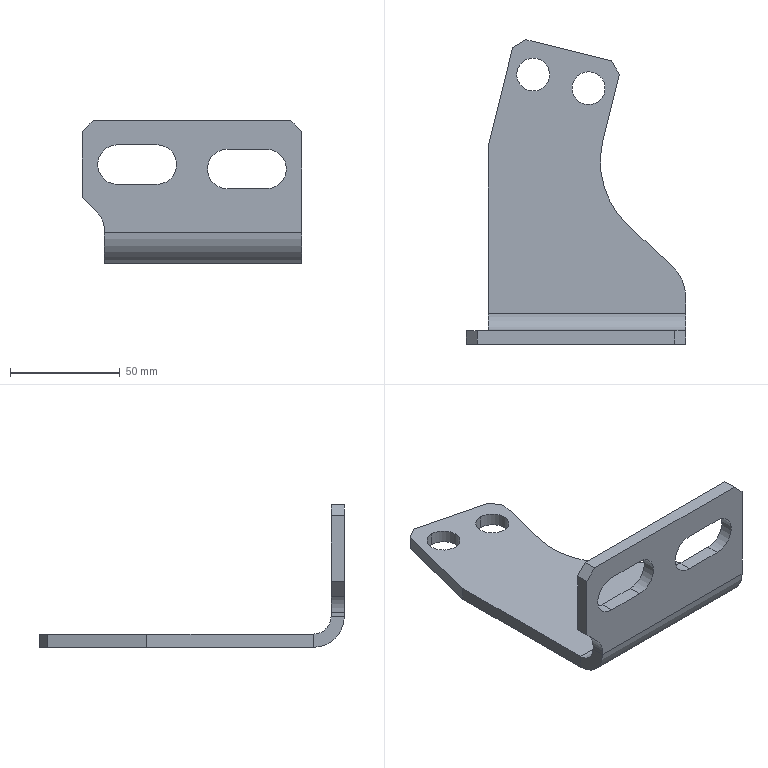Part | SolidWorks | features ICE 2, Chamfer 1, Fillet 1, FlatPattern 1, SMBaseFlange 1, SheetMetal 1 | 1 solid | 38 faces | box 100 x 138.801 x 65 mm | volume 74939 mm3 | plane 25 | cylinder 13 | commonest cylinder face diameters 15 x4 18 x4 16 x1 20 x1 28 x1 40 x1
STEP:
#1=CARTESIAN_POINT('',(5.761,-30.792,6.));
#2=VERTEX_POINT('',#1);
#3=CARTESIAN_POINT('',(5.761,-15.792,6.));
#4=VERTEX_POINT('',#3);
#5=CARTESIAN_POINT('',(5.761,-23.292,6.));
#6=DIRECTION('',(0.,0.,-1.));
#7=DIRECTION('',(0.,1.,0.));
#8=AXIS2_PLACEMENT_3D('',#5,#6,#7);
#9=CIRCLE('',#8,7.5);
#10=EDGE_CURVE('',#2,#4,#9,.T.);
#11=ORIENTED_EDGE('',*,*,#10,.F.);
#12=CARTESIAN_POINT('',(5.761,-30.792,0.));
#13=VERTEX_POINT('',#12);
#14=CARTESIAN_POINT('',(5.761,-30.792,0.));
#15=DIRECTION('',(0.,0.,-1.));
#16=VECTOR('',#15,1000.);
#17=LINE('',#14,#16);
#18=EDGE_CURVE('',#2,#13,#17,.T.);
#19=ORIENTED_EDGE('',*,*,#18,.T.);
#20=CARTESIAN_POINT('',(5.761,-15.792,0.));
#21=VERTEX_POINT('',#20);
#22=CARTESIAN_POINT('',(5.761,-23.292,0.));
#23=DIRECTION('',(0.,0.,-1.));
#24=DIRECTION('',(0.,1.,0.));
#25=AXIS2_PLACEMENT_3D('',#22,#23,#24);
#26=CIRCLE('',#25,7.5);
#27=EDGE_CURVE('',#13,#21,#26,.T.);
#28=ORIENTED_EDGE('',*,*,#27,.T.);
#29=CARTESIAN_POINT('',(5.761,-15.792,0.));
#30=DIRECTION('',(0.,0.,-1.));
#31=VECTOR('',#30,1000.);
#32=LINE('',#29,#31);
#33=EDGE_CURVE('',#4,#21,#32,.T.);
#34=ORIENTED_EDGE('',*,*,#33,.F.);
#35=EDGE_LOOP('',(#11,#19,#28,#34));
#36=FACE_OUTER_BOUND('',#35,.T.);
#37=CARTESIAN_POINT('',(5.761,-23.292,0.));
#38=DIRECTION('',(0.,0.,-1.));
#39=DIRECTION('',(0.,1.,0.));
#40=AXIS2_PLACEMENT_3D('',#37,#38,#39);
#41=CYLINDRICAL_SURFACE('',#40,7.5);
#42=ADVANCED_FACE('',(#36),#41,.F.);
#43=CARTESIAN_POINT('',(-19.481,-24.557,6.));
#44=VERTEX_POINT('',#43);
#45=CARTESIAN_POINT('',(-19.481,-9.557,6.));
#46=VERTEX_POINT('',#45);
#47=CARTESIAN_POINT('',(-19.481,-17.057,6.));
#48=DIRECTION('',(0.,0.,-1.));
#49=DIRECTION('',(0.,1.,0.));
#50=AXIS2_PLACEMENT_3D('',#47,#48,#49);
#51=CIRCLE('',#50,7.5);
#52=EDGE_CURVE('',#44,#46,#51,.T.);
#53=ORIENTED_EDGE('',*,*,#52,.F.);
#54=CARTESIAN_POINT('',(-19.481,-24.557,0.));
#55=VERTEX_POINT('',#54);
#56=CARTESIAN_POINT('',(-19.481,-24.557,0.));
#57=DIRECTION('',(0.,0.,-1.));
#58=VECTOR('',#57,1000.);
#59=LINE('',#56,#58);
#60=EDGE_CURVE('',#44,#55,#59,.T.);
#61=ORIENTED_EDGE('',*,*,#60,.T.);
#62=CARTESIAN_POINT('',(-19.481,-9.557,0.));
#63=VERTEX_POINT('',#62);
#64=CARTESIAN_POINT('',(-19.481,-17.057,0.));
#65=DIRECTION('',(0.,0.,-1.));
#66=DIRECTION('',(0.,1.,0.));
#67=AXIS2_PLACEMENT_3D('',#64,#65,#66);
#68=CIRCLE('',#67,7.5);
#69=EDGE_CURVE('',#55,#63,#68,.T.);
#70=ORIENTED_EDGE('',*,*,#69,.T.);
#71=CARTESIAN_POINT('',(-19.481,-9.557,0.));
#72=DIRECTION('',(0.,0.,-1.));
#73=VECTOR('',#72,1000.);
#74=LINE('',#71,#73);
#75=EDGE_CURVE('',#46,#63,#74,.T.);
#76=ORIENTED_EDGE('',*,*,#75,.F.);
#77=EDGE_LOOP('',(#53,#61,#70,#76));
#78=FACE_OUTER_BOUND('',#77,.T.);
#79=CARTESIAN_POINT('',(-19.481,-17.057,0.));
#80=DIRECTION('',(0.,0.,-1.));
#81=DIRECTION('',(0.,1.,0.));
#82=AXIS2_PLACEMENT_3D('',#79,#80,#81);
#83=CYLINDRICAL_SURFACE('',#82,7.5);
#84=ADVANCED_FACE('',(#78),#83,.F.);
#85=CARTESIAN_POINT('',(5.761,-23.292,0.));
#86=DIRECTION('',(0.,0.,-1.));
#87=DIRECTION('',(0.,1.,0.));
#88=AXIS2_PLACEMENT_3D('',#85,#86,#87);
#89=CIRCLE('',#88,7.5);
#90=EDGE_CURVE('',#21,#13,#89,.T.);
#91=ORIENTED_EDGE('',*,*,#90,.F.);
#92=ORIENTED_EDGE('',*,*,#27,.F.);
#93=EDGE_LOOP('',(#91,#92));
#94=FACE_BOUND('',#93,.T.);
#95=CARTESIAN_POINT('',(-19.481,-17.057,0.));
#96=DIRECTION('',(0.,0.,-1.));
#97=DIRECTION('',(0.,1.,0.));
#98=AXIS2_PLACEMENT_3D('',#95,#96,#97);
#99=CIRCLE('',#98,7.5);
#100=EDGE_CURVE('',#63,#55,#99,.T.);
#101=ORIENTED_EDGE('',*,*,#100,.F.);
#102=ORIENTED_EDGE('',*,*,#69,.F.);
#103=EDGE_LOOP('',(#101,#102));
#104=FACE_BOUND('',#103,.T.);
#105=CARTESIAN_POINT('',(-40.,-50.,0.));
#106=VERTEX_POINT('',#105);
#107=CARTESIAN_POINT('',(-28.847,-4.854,0.));
#108=VERTEX_POINT('',#107);
#109=CARTESIAN_POINT('',(-26.058,6.437,0.));
#110=DIRECTION('',(0.2398,0.9708,0.));
#111=VECTOR('',#110,1000.);
#112=LINE('',#109,#111);
#113=EDGE_CURVE('',#106,#108,#112,.T.);
#114=ORIENTED_EDGE('',*,*,#113,.T.);
#115=CARTESIAN_POINT('',(-22.794,-1.199,0.));
#116=VERTEX_POINT('',#115);
#117=CARTESIAN_POINT('',(31.082,31.332,0.));
#118=DIRECTION('',(0.8561,0.5169,0.));
#119=VECTOR('',#118,1000.);
#120=LINE('',#117,#119);
#121=EDGE_CURVE('',#108,#116,#120,.T.);
#122=ORIENTED_EDGE('',*,*,#121,.T.);
#123=CARTESIAN_POINT('',(16.074,-10.801,0.));
#124=VERTEX_POINT('',#123);
#125=CARTESIAN_POINT('',(-1.59,-6.437,0.));
#126=DIRECTION('',(0.9708,-0.2398,0.));
#127=VECTOR('',#126,1000.);
#128=LINE('',#125,#127);
#129=EDGE_CURVE('',#116,#124,#128,.T.);
#130=ORIENTED_EDGE('',*,*,#129,.T.);
#131=CARTESIAN_POINT('',(19.729,-16.854,0.));
#132=VERTEX_POINT('',#131);
#133=CARTESIAN_POINT('',(20.359,-17.897,0.));
#134=DIRECTION('',(0.5169,-0.8561,0.));
#135=VECTOR('',#134,1000.);
#136=LINE('',#133,#135);
#137=EDGE_CURVE('',#124,#132,#136,.T.);
#138=ORIENTED_EDGE('',*,*,#137,.T.);
#139=CARTESIAN_POINT('',(12.274,-47.03,0.));
#140=VERTEX_POINT('',#139);
#141=CARTESIAN_POINT('',(22.518,-5.563,0.));
#142=DIRECTION('',(-0.2398,-0.9708,0.));
#143=VECTOR('',#142,1000.);
#144=LINE('',#141,#143);
#145=EDGE_CURVE('',#132,#140,#144,.T.);
#146=ORIENTED_EDGE('',*,*,#145,.T.);
#147=CARTESIAN_POINT('',(23.998,-86.035,0.));
#148=VERTEX_POINT('',#147);
#149=CARTESIAN_POINT('',(51.107,-56.623,0.));
#150=DIRECTION('',(0.,0.,1.));
#151=DIRECTION('',(0.,1.,0.));
#152=AXIS2_PLACEMENT_3D('',#149,#150,#151);
#153=CIRCLE('',#152,40.);
#154=EDGE_CURVE('',#140,#148,#153,.T.);
#155=ORIENTED_EDGE('',*,*,#154,.T.);
#156=CARTESIAN_POINT('',(43.554,-104.059,0.));
#157=VERTEX_POINT('',#156);
#158=CARTESIAN_POINT('',(-31.852,-34.56,0.));
#159=DIRECTION('',(0.7353,-0.6777,0.));
#160=VECTOR('',#159,1000.);
#161=LINE('',#158,#160);
#162=EDGE_CURVE('',#148,#157,#161,.T.);
#163=ORIENTED_EDGE('',*,*,#162,.T.);
#164=CARTESIAN_POINT('',(50.,-118.766,0.));
#165=VERTEX_POINT('',#164);
#166=CARTESIAN_POINT('',(30.,-118.766,0.));
#167=DIRECTION('',(0.,0.,-1.));
#168=DIRECTION('',(0.,1.,0.));
#169=AXIS2_PLACEMENT_3D('',#166,#167,#168);
#170=CIRCLE('',#169,20.);
#171=EDGE_CURVE('',#157,#165,#170,.T.);
#172=ORIENTED_EDGE('',*,*,#171,.T.);
#173=CARTESIAN_POINT('',(50.,-126.,0.));
#174=VERTEX_POINT('',#173);
#175=CARTESIAN_POINT('',(50.,0.,0.));
#176=DIRECTION('',(0.,-1.,0.));
#177=VECTOR('',#176,1000.);
#178=LINE('',#175,#177);
#179=EDGE_CURVE('',#165,#174,#178,.T.);
#180=ORIENTED_EDGE('',*,*,#179,.T.);
#181=CARTESIAN_POINT('',(-40.,-126.,0.));
#182=VERTEX_POINT('',#181);
#183=CARTESIAN_POINT('',(50.,-126.,0.));
#184=DIRECTION('',(-1.,0.,0.));
#185=VECTOR('',#184,1000.);
#186=LINE('',#183,#185);
#187=EDGE_CURVE('',#174,#182,#186,.T.);
#188=ORIENTED_EDGE('',*,*,#187,.T.);
#189=CARTESIAN_POINT('',(-40.,-140.,0.));
#190=DIRECTION('',(0.,1.,0.));
#191=VECTOR('',#190,1000.);
#192=LINE('',#189,#191);
#193=EDGE_CURVE('',#182,#106,#192,.T.);
#194=ORIENTED_EDGE('',*,*,#193,.T.);
#195=EDGE_LOOP('',(#114,#122,#130,#138,#146,#155,#163,#172,#180,#188,#194));
#196=FACE_OUTER_BOUND('',#195,.T.);
#197=CARTESIAN_POINT('',(50.,0.,0.));
#198=DIRECTION('',(0.,0.,-1.));
#199=DIRECTION('',(0.,1.,0.));
#200=AXIS2_PLACEMENT_3D('',#197,#198,#199);
#201=PLANE('',#200);
#202=ADVANCED_FACE('',(#94,#104,#196),#201,.T.);
#203=CARTESIAN_POINT('',(-19.481,-17.057,6.));
#204=DIRECTION('',(0.,0.,-1.));
#205=DIRECTION('',(0.,1.,0.));
#206=AXIS2_PLACEMENT_3D('',#203,#204,#205);
#207=CIRCLE('',#206,7.5);
#208=EDGE_CURVE('',#46,#44,#207,.T.);
#209=ORIENTED_EDGE('',*,*,#208,.T.);
#210=ORIENTED_EDGE('',*,*,#52,.T.);
#211=EDGE_LOOP('',(#209,#210));
#212=FACE_BOUND('',#211,.T.);
#213=CARTESIAN_POINT('',(5.761,-23.292,6.));
#214=DIRECTION('',(0.,0.,-1.));
#215=DIRECTION('',(0.,1.,0.));
#216=AXIS2_PLACEMENT_3D('',#213,#214,#215);
#217=CIRCLE('',#216,7.5);
#218=EDGE_CURVE('',#4,#2,#217,.T.);
#219=ORIENTED_EDGE('',*,*,#218,.T.);
#220=ORIENTED_EDGE('',*,*,#10,.T.);
#221=EDGE_LOOP('',(#219,#220));
#222=FACE_BOUND('',#221,.T.);
#223=CARTESIAN_POINT('',(-22.794,-1.199,6.));
#224=VERTEX_POINT('',#223);
#225=CARTESIAN_POINT('',(16.074,-10.801,6.));
#226=VERTEX_POINT('',#225);
#227=CARTESIAN_POINT('',(-1.59,-6.437,6.));
#228=DIRECTION('',(0.9708,-0.2398,0.));
#229=VECTOR('',#228,1000.);
#230=LINE('',#227,#229);
#231=EDGE_CURVE('',#224,#226,#230,.T.);
#232=ORIENTED_EDGE('',*,*,#231,.F.);
#233=CARTESIAN_POINT('',(-28.847,-4.854,6.));
#234=VERTEX_POINT('',#233);
#235=CARTESIAN_POINT('',(-28.847,-4.854,6.));
#236=DIRECTION('',(-0.8561,-0.5169,0.));
#237=VECTOR('',#236,1000.);
#238=LINE('',#235,#237);
#239=EDGE_CURVE('',#224,#234,#238,.T.);
#240=ORIENTED_EDGE('',*,*,#239,.T.);
#241=CARTESIAN_POINT('',(-40.,-50.,6.));
#242=VERTEX_POINT('',#241);
#243=CARTESIAN_POINT('',(-26.058,6.437,6.));
#244=DIRECTION('',(0.2398,0.9708,0.));
#245=VECTOR('',#244,1000.);
#246=LINE('',#243,#245);
#247=EDGE_CURVE('',#242,#234,#246,.T.);
#248=ORIENTED_EDGE('',*,*,#247,.F.);
#249=CARTESIAN_POINT('',(-40.,-126.,6.));
#250=VERTEX_POINT('',#249);
#251=CARTESIAN_POINT('',(-40.,0.,6.));
#252=DIRECTION('',(0.,1.,0.));
#253=VECTOR('',#252,1000.);
#254=LINE('',#251,#253);
#255=EDGE_CURVE('',#250,#242,#254,.T.);
#256=ORIENTED_EDGE('',*,*,#255,.F.);
#257=CARTESIAN_POINT('',(50.,-126.,6.));
#258=VERTEX_POINT('',#257);
#259=CARTESIAN_POINT('',(50.,-126.,6.));
#260=DIRECTION('',(-1.,0.,0.));
#261=VECTOR('',#260,1000.);
#262=LINE('',#259,#261);
#263=EDGE_CURVE('',#258,#250,#262,.T.);
#264=ORIENTED_EDGE('',*,*,#263,.F.);
#265=CARTESIAN_POINT('',(50.,-118.766,6.));
#266=VERTEX_POINT('',#265);
#267=CARTESIAN_POINT('',(50.,0.,6.));
#268=DIRECTION('',(0.,-1.,0.));
#269=VECTOR('',#268,1000.);
#270=LINE('',#267,#269);
#271=EDGE_CURVE('',#266,#258,#270,.T.);
#272=ORIENTED_EDGE('',*,*,#271,.F.);
#273=CARTESIAN_POINT('',(43.554,-104.059,6.));
#274=VERTEX_POINT('',#273);
#275=CARTESIAN_POINT('',(30.,-118.766,6.));
#276=DIRECTION('',(0.,0.,1.));
#277=DIRECTION('',(0.,1.,0.));
#278=AXIS2_PLACEMENT_3D('',#275,#276,#277);
#279=CIRCLE('',#278,20.);
#280=EDGE_CURVE('',#266,#274,#279,.T.);
#281=ORIENTED_EDGE('',*,*,#280,.T.);
#282=CARTESIAN_POINT('',(23.998,-86.035,6.));
#283=VERTEX_POINT('',#282);
#284=CARTESIAN_POINT('',(-31.852,-34.56,6.));
#285=DIRECTION('',(0.7353,-0.6777,0.));
#286=VECTOR('',#285,1000.);
#287=LINE('',#284,#286);
#288=EDGE_CURVE('',#283,#274,#287,.T.);
#289=ORIENTED_EDGE('',*,*,#288,.F.);
#290=CARTESIAN_POINT('',(12.274,-47.03,6.));
#291=VERTEX_POINT('',#290);
#292=CARTESIAN_POINT('',(51.107,-56.623,6.));
#293=DIRECTION('',(0.,0.,1.));
#294=DIRECTION('',(0.,1.,0.));
#295=AXIS2_PLACEMENT_3D('',#292,#293,#294);
#296=CIRCLE('',#295,40.);
#297=EDGE_CURVE('',#291,#283,#296,.T.);
#298=ORIENTED_EDGE('',*,*,#297,.F.);
#299=CARTESIAN_POINT('',(19.729,-16.854,6.));
#300=VERTEX_POINT('',#299);
#301=CARTESIAN_POINT('',(22.518,-5.563,6.));
#302=DIRECTION('',(-0.2398,-0.9708,0.));
#303=VECTOR('',#302,1000.);
#304=LINE('',#301,#303);
#305=EDGE_CURVE('',#300,#291,#304,.T.);
#306=ORIENTED_EDGE('',*,*,#305,.F.);
#307=CARTESIAN_POINT('',(16.074,-10.801,6.));
#308=DIRECTION('',(-0.5169,0.8561,0.));
#309=VECTOR('',#308,1000.);
#310=LINE('',#307,#309);
#311=EDGE_CURVE('',#300,#226,#310,.T.);
#312=ORIENTED_EDGE('',*,*,#311,.T.);
#313=EDGE_LOOP('',(#232,#240,#248,#256,#264,#272,#281,#289,#298,#306,#312));
#314=FACE_OUTER_BOUND('',#313,.T.);
#315=CARTESIAN_POINT('',(50.,0.,6.));
#316=DIRECTION('',(0.,0.,-1.));
#317=DIRECTION('',(0.,1.,0.));
#318=AXIS2_PLACEMENT_3D('',#315,#316,#317);
#319=PLANE('',#318);
#320=ADVANCED_FACE('',(#212,#222,#314),#319,.F.);
#321=ORIENTED_EDGE('',*,*,#255,.T.);
#322=CARTESIAN_POINT('',(-40.,-50.,6.));
#323=DIRECTION('',(0.,0.,-1.));
#324=VECTOR('',#323,1000.);
#325=LINE('',#322,#324);
#326=EDGE_CURVE('',#242,#106,#325,.T.);
#327=ORIENTED_EDGE('',*,*,#326,.T.);
#328=ORIENTED_EDGE('',*,*,#193,.F.);
#329=CARTESIAN_POINT('',(-40.,-126.,0.));
#330=DIRECTION('',(0.,0.,1.));
#331=VECTOR('',#330,1000.);
#332=LINE('',#329,#331);
#333=EDGE_CURVE('',#182,#250,#332,.T.);
#334=ORIENTED_EDGE('',*,*,#333,.T.);
#335=EDGE_LOOP('',(#321,#327,#328,#334));
#336=FACE_OUTER_BOUND('',#335,.T.);
#337=CARTESIAN_POINT('',(-40.,-140.,0.));
#338=DIRECTION('',(-1.,0.,0.));
#339=DIRECTION('',(0.,1.,0.));
#340=AXIS2_PLACEMENT_3D('',#337,#338,#339);
#341=PLANE('',#340);
#342=ADVANCED_FACE('',(#336),#341,.T.);
#343=ORIENTED_EDGE('',*,*,#179,.F.);
#344=CARTESIAN_POINT('',(50.,-118.766,14.));
#345=DIRECTION('',(0.,0.,1.));
#346=VECTOR('',#345,1000.);
#347=LINE('',#344,#346);
#348=EDGE_CURVE('',#165,#266,#347,.T.);
#349=ORIENTED_EDGE('',*,*,#348,.T.);
#350=ORIENTED_EDGE('',*,*,#271,.T.);
#351=CARTESIAN_POINT('',(50.,-126.,6.));
#352=DIRECTION('',(0.,0.,-1.));
#353=VECTOR('',#352,1000.);
#354=LINE('',#351,#353);
#355=EDGE_CURVE('',#258,#174,#354,.T.);
#356=ORIENTED_EDGE('',*,*,#355,.T.);
#357=EDGE_LOOP('',(#343,#349,#350,#356));
#358=FACE_OUTER_BOUND('',#357,.T.);
#359=CARTESIAN_POINT('',(50.,-126.,14.));
#360=DIRECTION('',(1.,0.,0.));
#361=DIRECTION('',(0.,0.,-1.));
#362=AXIS2_PLACEMENT_3D('',#359,#360,#361);
#363=PLANE('',#362);
#364=ADVANCED_FACE('',(#358),#363,.T.);
#365=CARTESIAN_POINT('',(-50.,-134.,30.));
#366=VERTEX_POINT('',#365);
#367=CARTESIAN_POINT('',(-50.,-134.,60.));
#368=VERTEX_POINT('',#367);
#369=CARTESIAN_POINT('',(-50.,-134.,0.));
#370=DIRECTION('',(0.,0.,1.));
#371=VECTOR('',#370,1000.);
#372=LINE('',#369,#371);
#373=EDGE_CURVE('',#366,#368,#372,.T.);
#374=ORIENTED_EDGE('',*,*,#373,.T.);
#375=CARTESIAN_POINT('',(-45.,-134.,65.));
#376=VERTEX_POINT('',#375);
#377=CARTESIAN_POINT('',(-50.,-134.,60.));
#378=DIRECTION('',(0.7071,0.,0.7071));
#379=VECTOR('',#378,1000.);
#380=LINE('',#377,#379);
#381=EDGE_CURVE('',#368,#376,#380,.T.);
#382=ORIENTED_EDGE('',*,*,#381,.T.);
#383=CARTESIAN_POINT('',(45.,-134.,65.));
#384=VERTEX_POINT('',#383);
#385=CARTESIAN_POINT('',(50.,-134.,65.));
#386=DIRECTION('',(-1.,0.,0.));
#387=VECTOR('',#386,1000.);
#388=LINE('',#385,#387);
#389=EDGE_CURVE('',#384,#376,#388,.T.);
#390=ORIENTED_EDGE('',*,*,#389,.F.);
#391=CARTESIAN_POINT('',(50.,-134.,60.));
#392=VERTEX_POINT('',#391);
#393=CARTESIAN_POINT('',(45.,-134.,65.));
#394=DIRECTION('',(0.7071,0.,-0.7071));
#395=VECTOR('',#394,1000.);
#396=LINE('',#393,#395);
#397=EDGE_CURVE('',#384,#392,#396,.T.);
#398=ORIENTED_EDGE('',*,*,#397,.T.);
#399=CARTESIAN_POINT('',(50.,-134.,14.));
#400=VERTEX_POINT('',#399);
#401=CARTESIAN_POINT('',(50.,-134.,0.));
#402=DIRECTION('',(0.,0.,1.));
#403=VECTOR('',#402,1000.);
#404=LINE('',#401,#403);
#405=EDGE_CURVE('',#400,#392,#404,.T.);
#406=ORIENTED_EDGE('',*,*,#405,.F.);
#407=CARTESIAN_POINT('',(-40.,-134.,14.));
#408=VERTEX_POINT('',#407);
#409=CARTESIAN_POINT('',(50.,-134.,14.));
#410=DIRECTION('',(-1.,0.,0.));
#411=VECTOR('',#410,1000.);
#412=LINE('',#409,#411);
#413=EDGE_CURVE('',#400,#408,#412,.T.);
#414=ORIENTED_EDGE('',*,*,#413,.T.);
#415=CARTESIAN_POINT('',(-40.,-134.,15.858));
#416=VERTEX_POINT('',#415);
#417=CARTESIAN_POINT('',(-40.,-134.,0.));
#418=DIRECTION('',(0.,0.,1.));
#419=VECTOR('',#418,1000.);
#420=LINE('',#417,#419);
#421=EDGE_CURVE('',#408,#416,#420,.T.);
#422=ORIENTED_EDGE('',*,*,#421,.T.);
#423=CARTESIAN_POINT('',(-42.929,-134.,22.929));
#424=VERTEX_POINT('',#423);
#425=CARTESIAN_POINT('',(-50.,-134.,15.858));
#426=DIRECTION('',(0.,-1.,0.));
#427=DIRECTION('',(0.,0.,-1.));
#428=AXIS2_PLACEMENT_3D('',#425,#426,#427);
#429=CIRCLE('',#428,10.);
#430=EDGE_CURVE('',#416,#424,#429,.T.);
#431=ORIENTED_EDGE('',*,*,#430,.T.);
#432=CARTESIAN_POINT('',(15.,-134.,-35.));
#433=DIRECTION('',(-0.7071,0.,0.7071));
#434=VECTOR('',#433,1000.);
#435=LINE('',#432,#434);
#436=EDGE_CURVE('',#424,#366,#435,.T.);
#437=ORIENTED_EDGE('',*,*,#436,.T.);
#438=EDGE_LOOP('',(#374,#382,#390,#398,#406,#414,#422,#431,#437));
#439=FACE_OUTER_BOUND('',#438,.T.);
#440=CARTESIAN_POINT('',(-34.,-134.,54.));
#441=VERTEX_POINT('',#440);
#442=CARTESIAN_POINT('',(-34.,-134.,36.));
#443=VERTEX_POINT('',#442);
#444=CARTESIAN_POINT('',(-34.,-134.,45.));
#445=DIRECTION('',(0.,-1.,0.));
#446=DIRECTION('',(0.,0.,-1.));
#447=AXIS2_PLACEMENT_3D('',#444,#445,#446);
#448=CIRCLE('',#447,9.);
#449=EDGE_CURVE('',#441,#443,#448,.T.);
#450=ORIENTED_EDGE('',*,*,#449,.T.);
#451=CARTESIAN_POINT('',(-16.,-134.,36.));
#452=VERTEX_POINT('',#451);
#453=CARTESIAN_POINT('',(50.,-134.,36.));
#454=DIRECTION('',(1.,0.,0.));
#455=VECTOR('',#454,1000.);
#456=LINE('',#453,#455);
#457=EDGE_CURVE('',#443,#452,#456,.T.);
#458=ORIENTED_EDGE('',*,*,#457,.T.);
#459=CARTESIAN_POINT('',(-16.,-134.,54.));
#460=VERTEX_POINT('',#459);
#461=CARTESIAN_POINT('',(-16.,-134.,45.));
#462=DIRECTION('',(0.,-1.,0.));
#463=DIRECTION('',(0.,0.,-1.));
#464=AXIS2_PLACEMENT_3D('',#461,#462,#463);
#465=CIRCLE('',#464,9.);
#466=EDGE_CURVE('',#452,#460,#465,.T.);
#467=ORIENTED_EDGE('',*,*,#466,.T.);
#468=CARTESIAN_POINT('',(50.,-134.,54.));
#469=DIRECTION('',(-1.,0.,0.));
#470=VECTOR('',#469,1000.);
#471=LINE('',#468,#470);
#472=EDGE_CURVE('',#460,#441,#471,.T.);
#473=ORIENTED_EDGE('',*,*,#472,.T.);
#474=EDGE_LOOP('',(#450,#458,#467,#473));
#475=FACE_BOUND('',#474,.T.);
#476=CARTESIAN_POINT('',(16.,-134.,52.));
#477=VERTEX_POINT('',#476);
#478=CARTESIAN_POINT('',(16.,-134.,34.));
#479=VERTEX_POINT('',#478);
#480=CARTESIAN_POINT('',(16.,-134.,43.));
#481=DIRECTION('',(0.,-1.,0.));
#482=DIRECTION('',(0.,0.,-1.));
#483=AXIS2_PLACEMENT_3D('',#480,#481,#482);
#484=CIRCLE('',#483,9.);
#485=EDGE_CURVE('',#477,#479,#484,.T.);
#486=ORIENTED_EDGE('',*,*,#485,.T.);
#487=CARTESIAN_POINT('',(34.,-134.,34.));
#488=VERTEX_POINT('',#487);
#489=CARTESIAN_POINT('',(50.,-134.,34.));
#490=DIRECTION('',(1.,0.,0.));
#491=VECTOR('',#490,1000.);
#492=LINE('',#489,#491);
#493=EDGE_CURVE('',#479,#488,#492,.T.);
#494=ORIENTED_EDGE('',*,*,#493,.T.);
#495=CARTESIAN_POINT('',(34.,-134.,52.));
#496=VERTEX_POINT('',#495);
#497=CARTESIAN_POINT('',(34.,-134.,43.));
#498=DIRECTION('',(0.,-1.,0.));
#499=DIRECTION('',(0.,0.,-1.));
#500=AXIS2_PLACEMENT_3D('',#497,#498,#499);
#501=CIRCLE('',#500,9.);
#502=EDGE_CURVE('',#488,#496,#501,.T.);
#503=ORIENTED_EDGE('',*,*,#502,.T.);
#504=CARTESIAN_POINT('',(50.,-134.,52.));
#505=DIRECTION('',(-1.,0.,0.));
#506=VECTOR('',#505,1000.);
#507=LINE('',#504,#506);
#508=EDGE_CURVE('',#496,#477,#507,.T.);
#509=ORIENTED_EDGE('',*,*,#508,.T.);
#510=EDGE_LOOP('',(#486,#494,#503,#509));
#511=FACE_BOUND('',#510,.T.);
#512=CARTESIAN_POINT('',(50.,-134.,0.));
#513=DIRECTION('',(0.,-1.,0.));
#514=DIRECTION('',(0.,0.,-1.));
#515=AXIS2_PLACEMENT_3D('',#512,#513,#514);
#516=PLANE('',#515);
#517=ADVANCED_FACE('',(#439,#475,#511),#516,.F.);
#518=CARTESIAN_POINT('',(-34.,-140.,36.));
#519=VERTEX_POINT('',#518);
#520=CARTESIAN_POINT('',(-16.,-140.,36.));
#521=VERTEX_POINT('',#520);
#522=CARTESIAN_POINT('',(50.,-140.,36.));
#523=DIRECTION('',(1.,0.,0.));
#524=VECTOR('',#523,1000.);
#525=LINE('',#522,#524);
#526=EDGE_CURVE('',#519,#521,#525,.T.);
#527=ORIENTED_EDGE('',*,*,#526,.F.);
#528=CARTESIAN_POINT('',(-34.,-140.,54.));
#529=VERTEX_POINT('',#528);
#530=CARTESIAN_POINT('',(-34.,-140.,45.));
#531=DIRECTION('',(0.,-1.,0.));
#532=DIRECTION('',(0.,0.,-1.));
#533=AXIS2_PLACEMENT_3D('',#530,#531,#532);
#534=CIRCLE('',#533,9.);
#535=EDGE_CURVE('',#529,#519,#534,.T.);
#536=ORIENTED_EDGE('',*,*,#535,.F.);
#537=CARTESIAN_POINT('',(-16.,-140.,54.));
#538=VERTEX_POINT('',#537);
#539=CARTESIAN_POINT('',(50.,-140.,54.));
#540=DIRECTION('',(-1.,0.,0.));
#541=VECTOR('',#540,1000.);
#542=LINE('',#539,#541);
#543=EDGE_CURVE('',#538,#529,#542,.T.);
#544=ORIENTED_EDGE('',*,*,#543,.F.);
#545=CARTESIAN_POINT('',(-16.,-140.,45.));
#546=DIRECTION('',(0.,-1.,0.));
#547=DIRECTION('',(0.,0.,-1.));
#548=AXIS2_PLACEMENT_3D('',#545,#546,#547);
#549=CIRCLE('',#548,9.);
#550=EDGE_CURVE('',#521,#538,#549,.T.);
#551=ORIENTED_EDGE('',*,*,#550,.F.);
#552=EDGE_LOOP('',(#527,#536,#544,#551));
#553=FACE_BOUND('',#552,.T.);
#554=CARTESIAN_POINT('',(45.,-140.,65.));
#555=VERTEX_POINT('',#554);
#556=CARTESIAN_POINT('',(-45.,-140.,65.));
#557=VERTEX_POINT('',#556);
#558=CARTESIAN_POINT('',(50.,-140.,65.));
#559=DIRECTION('',(-1.,0.,0.));
#560=VECTOR('',#559,1000.);
#561=LINE('',#558,#560);
#562=EDGE_CURVE('',#555,#557,#561,.T.);
#563=ORIENTED_EDGE('',*,*,#562,.T.);
#564=CARTESIAN_POINT('',(-50.,-140.,60.));
#565=VERTEX_POINT('',#564);
#566=CARTESIAN_POINT('',(-30.,-140.,80.));
#567=DIRECTION('',(-0.7071,0.,-0.7071));
#568=VECTOR('',#567,1000.);
#569=LINE('',#566,#568);
#570=EDGE_CURVE('',#557,#565,#569,.T.);
#571=ORIENTED_EDGE('',*,*,#570,.T.);
#572=CARTESIAN_POINT('',(-50.,-140.,30.));
#573=VERTEX_POINT('',#572);
#574=CARTESIAN_POINT('',(-50.,-140.,0.));
#575=DIRECTION('',(0.,0.,1.));
#576=VECTOR('',#575,1000.);
#577=LINE('',#574,#576);
#578=EDGE_CURVE('',#573,#565,#577,.T.);
#579=ORIENTED_EDGE('',*,*,#578,.F.);
#580=CARTESIAN_POINT('',(-42.929,-140.,22.929));
#581=VERTEX_POINT('',#580);
#582=CARTESIAN_POINT('',(15.,-140.,-35.));
#583=DIRECTION('',(-0.7071,0.,0.7071));
#584=VECTOR('',#583,1000.);
#585=LINE('',#582,#584);
#586=EDGE_CURVE('',#581,#573,#585,.T.);
#587=ORIENTED_EDGE('',*,*,#586,.F.);
#588=CARTESIAN_POINT('',(-40.,-140.,15.858));
#589=VERTEX_POINT('',#588);
#590=CARTESIAN_POINT('',(-50.,-140.,15.858));
#591=DIRECTION('',(0.,-1.,0.));
#592=DIRECTION('',(0.,0.,-1.));
#593=AXIS2_PLACEMENT_3D('',#590,#591,#592);
#594=CIRCLE('',#593,10.);
#595=EDGE_CURVE('',#589,#581,#594,.T.);
#596=ORIENTED_EDGE('',*,*,#595,.F.);
#597=CARTESIAN_POINT('',(-40.,-140.,14.));
#598=VERTEX_POINT('',#597);
#599=CARTESIAN_POINT('',(-40.,-140.,0.));
#600=DIRECTION('',(0.,0.,1.));
#601=VECTOR('',#600,1000.);
#602=LINE('',#599,#601);
#603=EDGE_CURVE('',#598,#589,#602,.T.);
#604=ORIENTED_EDGE('',*,*,#603,.F.);
#605=CARTESIAN_POINT('',(50.,-140.,14.));
#606=VERTEX_POINT('',#605);
#607=CARTESIAN_POINT('',(50.,-140.,14.));
#608=DIRECTION('',(-1.,0.,0.));
#609=VECTOR('',#608,1000.);
#610=LINE('',#607,#609);
#611=EDGE_CURVE('',#606,#598,#610,.T.);
#612=ORIENTED_EDGE('',*,*,#611,.F.);
#613=CARTESIAN_POINT('',(50.,-140.,60.));
#614=VERTEX_POINT('',#613);
#615=CARTESIAN_POINT('',(50.,-140.,0.));
#616=DIRECTION('',(0.,0.,1.));
#617=VECTOR('',#616,1000.);
#618=LINE('',#615,#617);
#619=EDGE_CURVE('',#606,#614,#618,.T.);
#620=ORIENTED_EDGE('',*,*,#619,.T.);
#621=CARTESIAN_POINT('',(80.,-140.,30.));
#622=DIRECTION('',(-0.7071,0.,0.7071));
#623=VECTOR('',#622,1000.);
#624=LINE('',#621,#623);
#625=EDGE_CURVE('',#614,#555,#624,.T.);
#626=ORIENTED_EDGE('',*,*,#625,.T.);
#627=EDGE_LOOP('',(#563,#571,#579,#587,#596,#604,#612,#620,#626));
#628=FACE_OUTER_BOUND('',#627,.T.);
#629=CARTESIAN_POINT('',(16.,-140.,34.));
#630=VERTEX_POINT('',#629);
#631=CARTESIAN_POINT('',(34.,-140.,34.));
#632=VERTEX_POINT('',#631);
#633=CARTESIAN_POINT('',(50.,-140.,34.));
#634=DIRECTION('',(1.,0.,0.));
#635=VECTOR('',#634,1000.);
#636=LINE('',#633,#635);
#637=EDGE_CURVE('',#630,#632,#636,.T.);
#638=ORIENTED_EDGE('',*,*,#637,.F.);
#639=CARTESIAN_POINT('',(16.,-140.,52.));
#640=VERTEX_POINT('',#639);
#641=CARTESIAN_POINT('',(16.,-140.,43.));
#642=DIRECTION('',(0.,-1.,0.));
#643=DIRECTION('',(0.,0.,-1.));
#644=AXIS2_PLACEMENT_3D('',#641,#642,#643);
#645=CIRCLE('',#644,9.);
#646=EDGE_CURVE('',#640,#630,#645,.T.);
#647=ORIENTED_EDGE('',*,*,#646,.F.);
#648=CARTESIAN_POINT('',(34.,-140.,52.));
#649=VERTEX_POINT('',#648);
#650=CARTESIAN_POINT('',(50.,-140.,52.));
#651=DIRECTION('',(-1.,0.,0.));
#652=VECTOR('',#651,1000.);
#653=LINE('',#650,#652);
#654=EDGE_CURVE('',#649,#640,#653,.T.);
#655=ORIENTED_EDGE('',*,*,#654,.F.);
#656=CARTESIAN_POINT('',(34.,-140.,43.));
#657=DIRECTION('',(0.,-1.,0.));
#658=DIRECTION('',(0.,0.,-1.));
#659=AXIS2_PLACEMENT_3D('',#656,#657,#658);
#660=CIRCLE('',#659,9.);
#661=EDGE_CURVE('',#632,#649,#660,.T.);
#662=ORIENTED_EDGE('',*,*,#661,.F.);
#663=EDGE_LOOP('',(#638,#647,#655,#662));
#664=FACE_BOUND('',#663,.T.);
#665=CARTESIAN_POINT('',(50.,-140.,0.));
#666=DIRECTION('',(0.,-1.,0.));
#667=DIRECTION('',(0.,0.,-1.));
#668=AXIS2_PLACEMENT_3D('',#665,#666,#667);
#669=PLANE('',#668);
#670=ADVANCED_FACE('',(#553,#628,#664),#669,.T.);
#671=ORIENTED_EDGE('',*,*,#611,.T.);
#672=CARTESIAN_POINT('',(-40.,-126.,14.));
#673=DIRECTION('',(-1.,0.,0.));
#674=DIRECTION('',(0.,0.,-1.));
#675=AXIS2_PLACEMENT_3D('',#672,#673,#674);
#676=CIRCLE('',#675,14.);
#677=EDGE_CURVE('',#182,#598,#676,.T.);
#678=ORIENTED_EDGE('',*,*,#677,.F.);
#679=ORIENTED_EDGE('',*,*,#187,.F.);
#680=CARTESIAN_POINT('',(50.,-126.,14.));
#681=DIRECTION('',(-1.,0.,0.));
#682=DIRECTION('',(0.,0.,-1.));
#683=AXIS2_PLACEMENT_3D('',#680,#681,#682);
#684=CIRCLE('',#683,14.);
#685=EDGE_CURVE('',#174,#606,#684,.T.);
#686=ORIENTED_EDGE('',*,*,#685,.T.);
#687=EDGE_LOOP('',(#671,#678,#679,#686));
#688=FACE_OUTER_BOUND('',#687,.T.);
#689=CARTESIAN_POINT('',(50.,-126.,14.));
#690=DIRECTION('',(-1.,0.,0.));
#691=DIRECTION('',(0.,0.,1.));
#692=AXIS2_PLACEMENT_3D('',#689,#690,#691);
#693=CYLINDRICAL_SURFACE('',#692,14.);
#694=ADVANCED_FACE('',(#688),#693,.T.);
#695=CARTESIAN_POINT('',(-40.,-126.,14.));
#696=DIRECTION('',(-1.,0.,0.));
#697=DIRECTION('',(0.,0.,1.));
#698=AXIS2_PLACEMENT_3D('',#695,#696,#697);
#699=CIRCLE('',#698,8.);
#700=EDGE_CURVE('',#250,#408,#699,.T.);
#701=ORIENTED_EDGE('',*,*,#700,.T.);
#702=ORIENTED_EDGE('',*,*,#413,.F.);
#703=CARTESIAN_POINT('',(50.,-126.,14.));
#704=DIRECTION('',(-1.,0.,0.));
#705=DIRECTION('',(0.,0.,-1.));
#706=AXIS2_PLACEMENT_3D('',#703,#704,#705);
#707=CIRCLE('',#706,8.);
#708=EDGE_CURVE('',#258,#400,#707,.T.);
#709=ORIENTED_EDGE('',*,*,#708,.F.);
#710=ORIENTED_EDGE('',*,*,#263,.T.);
#711=EDGE_LOOP('',(#701,#702,#709,#710));
#712=FACE_OUTER_BOUND('',#711,.T.);
#713=CARTESIAN_POINT('',(50.,-126.,14.));
#714=DIRECTION('',(-1.,0.,0.));
#715=DIRECTION('',(0.,0.,1.));
#716=AXIS2_PLACEMENT_3D('',#713,#714,#715);
#717=CYLINDRICAL_SURFACE('',#716,8.);
#718=ADVANCED_FACE('',(#712),#717,.F.);
#719=ORIENTED_EDGE('',*,*,#578,.T.);
#720=CARTESIAN_POINT('',(-50.,-134.,60.));
#721=DIRECTION('',(0.,1.,0.));
#722=VECTOR('',#721,1000.);
#723=LINE('',#720,#722);
#724=EDGE_CURVE('',#565,#368,#723,.T.);
#725=ORIENTED_EDGE('',*,*,#724,.T.);
#726=ORIENTED_EDGE('',*,*,#373,.F.);
#727=CARTESIAN_POINT('',(-50.,-134.,30.));
#728=DIRECTION('',(0.,-1.,0.));
#729=VECTOR('',#728,1000.);
#730=LINE('',#727,#729);
#731=EDGE_CURVE('',#366,#573,#730,.T.);
#732=ORIENTED_EDGE('',*,*,#731,.T.);
#733=EDGE_LOOP('',(#719,#725,#726,#732));
#734=FACE_OUTER_BOUND('',#733,.T.);
#735=CARTESIAN_POINT('',(-50.,-126.,14.));
#736=DIRECTION('',(1.,0.,0.));
#737=DIRECTION('',(0.,0.,-1.));
#738=AXIS2_PLACEMENT_3D('',#735,#736,#737);
#739=PLANE('',#738);
#740=ADVANCED_FACE('',(#734),#739,.F.);
#741=CARTESIAN_POINT('',(50.,-140.,14.));
#742=DIRECTION('',(0.,1.,0.));
#743=VECTOR('',#742,1000.);
#744=LINE('',#741,#743);
#745=EDGE_CURVE('',#606,#400,#744,.T.);
#746=ORIENTED_EDGE('',*,*,#745,.F.);
#747=ORIENTED_EDGE('',*,*,#685,.F.);
#748=ORIENTED_EDGE('',*,*,#355,.F.);
#749=ORIENTED_EDGE('',*,*,#708,.T.);
#750=EDGE_LOOP('',(#746,#747,#748,#749));
#751=FACE_OUTER_BOUND('',#750,.T.);
#752=CARTESIAN_POINT('',(50.,-140.,14.));
#753=DIRECTION('',(1.,0.,0.));
#754=DIRECTION('',(0.,0.,-1.));
#755=AXIS2_PLACEMENT_3D('',#752,#753,#754);
#756=PLANE('',#755);
#757=ADVANCED_FACE('',(#751),#756,.T.);
#758=ORIENTED_EDGE('',*,*,#405,.T.);
#759=CARTESIAN_POINT('',(50.,-126.,60.));
#760=DIRECTION('',(0.,-1.,0.));
#761=VECTOR('',#760,1000.);
#762=LINE('',#759,#761);
#763=EDGE_CURVE('',#392,#614,#762,.T.);
#764=ORIENTED_EDGE('',*,*,#763,.T.);
#765=ORIENTED_EDGE('',*,*,#619,.F.);
#766=ORIENTED_EDGE('',*,*,#745,.T.);
#767=EDGE_LOOP('',(#758,#764,#765,#766));
#768=FACE_OUTER_BOUND('',#767,.T.);
#769=CARTESIAN_POINT('',(50.,-126.,6.));
#770=DIRECTION('',(1.,0.,0.));
#771=DIRECTION('',(0.,0.,-1.));
#772=AXIS2_PLACEMENT_3D('',#769,#770,#771);
#773=PLANE('',#772);
#774=ADVANCED_FACE('',(#768),#773,.T.);
#775=ORIENTED_EDGE('',*,*,#389,.T.);
#776=CARTESIAN_POINT('',(-45.,-140.,65.));
#777=DIRECTION('',(0.,-1.,0.));
#778=VECTOR('',#777,1000.);
#779=LINE('',#776,#778);
#780=EDGE_CURVE('',#376,#557,#779,.T.);
#781=ORIENTED_EDGE('',*,*,#780,.T.);
#782=ORIENTED_EDGE('',*,*,#562,.F.);
#783=CARTESIAN_POINT('',(45.,-140.,65.));
#784=DIRECTION('',(0.,1.,0.));
#785=VECTOR('',#784,1000.);
#786=LINE('',#783,#785);
#787=EDGE_CURVE('',#555,#384,#786,.T.);
#788=ORIENTED_EDGE('',*,*,#787,.T.);
#789=EDGE_LOOP('',(#775,#781,#782,#788));
#790=FACE_OUTER_BOUND('',#789,.T.);
#791=CARTESIAN_POINT('',(50.,-140.,65.));
#792=DIRECTION('',(0.,0.,1.));
#793=DIRECTION('',(1.,0.,0.));
#794=AXIS2_PLACEMENT_3D('',#791,#792,#793);
#795=PLANE('',#794);
#796=ADVANCED_FACE('',(#790),#795,.T.);
#797=ORIENTED_EDGE('',*,*,#731,.F.);
#798=ORIENTED_EDGE('',*,*,#436,.F.);
#799=CARTESIAN_POINT('',(-42.929,-134.,22.929));
#800=DIRECTION('',(0.,-1.,0.));
#801=VECTOR('',#800,1000.);
#802=LINE('',#799,#801);
#803=EDGE_CURVE('',#424,#581,#802,.T.);
#804=ORIENTED_EDGE('',*,*,#803,.T.);
#805=ORIENTED_EDGE('',*,*,#586,.T.);
#806=EDGE_LOOP('',(#797,#798,#804,#805));
#807=FACE_OUTER_BOUND('',#806,.T.);
#808=CARTESIAN_POINT('',(15.,-134.,-35.));
#809=DIRECTION('',(0.7071,0.,0.7071));
#810=DIRECTION('',(-0.7071,0.,0.7071));
#811=AXIS2_PLACEMENT_3D('',#808,#809,#810);
#812=PLANE('',#811);
#813=ADVANCED_FACE('',(#807),#812,.F.);
#814=ORIENTED_EDGE('',*,*,#803,.F.);
#815=ORIENTED_EDGE('',*,*,#430,.F.);
#816=CARTESIAN_POINT('',(-40.,-134.,15.858));
#817=DIRECTION('',(0.,-1.,0.));
#818=VECTOR('',#817,1000.);
#819=LINE('',#816,#818);
#820=EDGE_CURVE('',#416,#589,#819,.T.);
#821=ORIENTED_EDGE('',*,*,#820,.T.);
#822=ORIENTED_EDGE('',*,*,#595,.T.);
#823=EDGE_LOOP('',(#814,#815,#821,#822));
#824=FACE_OUTER_BOUND('',#823,.T.);
#825=CARTESIAN_POINT('',(-50.,-134.,15.858));
#826=DIRECTION('',(0.,-1.,0.));
#827=DIRECTION('',(0.,0.,-1.));
#828=AXIS2_PLACEMENT_3D('',#825,#826,#827);
#829=CYLINDRICAL_SURFACE('',#828,10.);
#830=ADVANCED_FACE('',(#824),#829,.F.);
#831=ORIENTED_EDGE('',*,*,#820,.F.);
#832=ORIENTED_EDGE('',*,*,#421,.F.);
#833=CARTESIAN_POINT('',(-40.,-134.,14.));
#834=DIRECTION('',(0.,-1.,0.));
#835=VECTOR('',#834,1000.);
#836=LINE('',#833,#835);
#837=EDGE_CURVE('',#408,#598,#836,.T.);
#838=ORIENTED_EDGE('',*,*,#837,.T.);
#839=ORIENTED_EDGE('',*,*,#603,.T.);
#840=EDGE_LOOP('',(#831,#832,#838,#839));
#841=FACE_OUTER_BOUND('',#840,.T.);
#842=CARTESIAN_POINT('',(-40.,-134.,0.));
#843=DIRECTION('',(1.,0.,0.));
#844=DIRECTION('',(0.,0.,1.));
#845=AXIS2_PLACEMENT_3D('',#842,#843,#844);
#846=PLANE('',#845);
#847=ADVANCED_FACE('',(#841),#846,.F.);
#848=ORIENTED_EDGE('',*,*,#677,.T.);
#849=ORIENTED_EDGE('',*,*,#837,.F.);
#850=ORIENTED_EDGE('',*,*,#700,.F.);
#851=ORIENTED_EDGE('',*,*,#333,.F.);
#852=EDGE_LOOP('',(#848,#849,#850,#851));
#853=FACE_OUTER_BOUND('',#852,.T.);
#854=CARTESIAN_POINT('',(-40.,-126.,14.));
#855=DIRECTION('',(-1.,0.,0.));
#856=DIRECTION('',(0.,0.,1.));
#857=AXIS2_PLACEMENT_3D('',#854,#855,#856);
#858=PLANE('',#857);
#859=ADVANCED_FACE('',(#853),#858,.T.);
#860=CARTESIAN_POINT('',(-34.,-134.,36.));
#861=DIRECTION('',(0.,-1.,0.));
#862=VECTOR('',#861,1000.);
#863=LINE('',#860,#862);
#864=EDGE_CURVE('',#443,#519,#863,.T.);
#865=ORIENTED_EDGE('',*,*,#864,.F.);
#866=ORIENTED_EDGE('',*,*,#449,.F.);
#867=CARTESIAN_POINT('',(-34.,-134.,54.));
#868=DIRECTION('',(0.,-1.,0.));
#869=VECTOR('',#868,1000.);
#870=LINE('',#867,#869);
#871=EDGE_CURVE('',#441,#529,#870,.T.);
#872=ORIENTED_EDGE('',*,*,#871,.T.);
#873=ORIENTED_EDGE('',*,*,#535,.T.);
#874=EDGE_LOOP('',(#865,#866,#872,#873));
#875=FACE_OUTER_BOUND('',#874,.T.);
#876=CARTESIAN_POINT('',(-34.,-134.,45.));
#877=DIRECTION('',(0.,-1.,0.));
#878=DIRECTION('',(0.,0.,-1.));
#879=AXIS2_PLACEMENT_3D('',#876,#877,#878);
#880=CYLINDRICAL_SURFACE('',#879,9.);
#881=ADVANCED_FACE('',(#875),#880,.F.);
#882=ORIENTED_EDGE('',*,*,#871,.F.);
#883=ORIENTED_EDGE('',*,*,#472,.F.);
#884=CARTESIAN_POINT('',(-16.,-134.,54.));
#885=DIRECTION('',(0.,-1.,0.));
#886=VECTOR('',#885,1000.);
#887=LINE('',#884,#886);
#888=EDGE_CURVE('',#460,#538,#887,.T.);
#889=ORIENTED_EDGE('',*,*,#888,.T.);
#890=ORIENTED_EDGE('',*,*,#543,.T.);
#891=EDGE_LOOP('',(#882,#883,#889,#890));
#892=FACE_OUTER_BOUND('',#891,.T.);
#893=CARTESIAN_POINT('',(50.,-134.,54.));
#894=DIRECTION('',(0.,0.,1.));
#895=DIRECTION('',(-1.,0.,0.));
#896=AXIS2_PLACEMENT_3D('',#893,#894,#895);
#897=PLANE('',#896);
#898=ADVANCED_FACE('',(#892),#897,.F.);
#899=ORIENTED_EDGE('',*,*,#888,.F.);
#900=ORIENTED_EDGE('',*,*,#466,.F.);
#901=CARTESIAN_POINT('',(-16.,-134.,36.));
#902=DIRECTION('',(0.,-1.,0.));
#903=VECTOR('',#902,1000.);
#904=LINE('',#901,#903);
#905=EDGE_CURVE('',#452,#521,#904,.T.);
#906=ORIENTED_EDGE('',*,*,#905,.T.);
#907=ORIENTED_EDGE('',*,*,#550,.T.);
#908=EDGE_LOOP('',(#899,#900,#906,#907));
#909=FACE_OUTER_BOUND('',#908,.T.);
#910=CARTESIAN_POINT('',(-16.,-134.,45.));
#911=DIRECTION('',(0.,-1.,0.));
#912=DIRECTION('',(0.,0.,-1.));
#913=AXIS2_PLACEMENT_3D('',#910,#911,#912);
#914=CYLINDRICAL_SURFACE('',#913,9.);
#915=ADVANCED_FACE('',(#909),#914,.F.);
#916=ORIENTED_EDGE('',*,*,#457,.F.);
#917=ORIENTED_EDGE('',*,*,#864,.T.);
#918=ORIENTED_EDGE('',*,*,#526,.T.);
#919=ORIENTED_EDGE('',*,*,#905,.F.);
#920=EDGE_LOOP('',(#916,#917,#918,#919));
#921=FACE_OUTER_BOUND('',#920,.T.);
#922=CARTESIAN_POINT('',(50.,-134.,36.));
#923=DIRECTION('',(0.,0.,-1.));
#924=DIRECTION('',(1.,0.,0.));
#925=AXIS2_PLACEMENT_3D('',#922,#923,#924);
#926=PLANE('',#925);
#927=ADVANCED_FACE('',(#921),#926,.F.);
#928=CARTESIAN_POINT('',(16.,-134.,34.));
#929=DIRECTION('',(0.,-1.,0.));
#930=VECTOR('',#929,1000.);
#931=LINE('',#928,#930);
#932=EDGE_CURVE('',#479,#630,#931,.T.);
#933=ORIENTED_EDGE('',*,*,#932,.F.);
#934=ORIENTED_EDGE('',*,*,#485,.F.);
#935=CARTESIAN_POINT('',(16.,-134.,52.));
#936=DIRECTION('',(0.,-1.,0.));
#937=VECTOR('',#936,1000.);
#938=LINE('',#935,#937);
#939=EDGE_CURVE('',#477,#640,#938,.T.);
#940=ORIENTED_EDGE('',*,*,#939,.T.);
#941=ORIENTED_EDGE('',*,*,#646,.T.);
#942=EDGE_LOOP('',(#933,#934,#940,#941));
#943=FACE_OUTER_BOUND('',#942,.T.);
#944=CARTESIAN_POINT('',(16.,-134.,43.));
#945=DIRECTION('',(0.,-1.,0.));
#946=DIRECTION('',(0.,0.,-1.));
#947=AXIS2_PLACEMENT_3D('',#944,#945,#946);
#948=CYLINDRICAL_SURFACE('',#947,9.);
#949=ADVANCED_FACE('',(#943),#948,.F.);
#950=ORIENTED_EDGE('',*,*,#939,.F.);
#951=ORIENTED_EDGE('',*,*,#508,.F.);
#952=CARTESIAN_POINT('',(34.,-134.,52.));
#953=DIRECTION('',(0.,-1.,0.));
#954=VECTOR('',#953,1000.);
#955=LINE('',#952,#954);
#956=EDGE_CURVE('',#496,#649,#955,.T.);
#957=ORIENTED_EDGE('',*,*,#956,.T.);
#958=ORIENTED_EDGE('',*,*,#654,.T.);
#959=EDGE_LOOP('',(#950,#951,#957,#958));
#960=FACE_OUTER_BOUND('',#959,.T.);
#961=CARTESIAN_POINT('',(50.,-134.,52.));
#962=DIRECTION('',(0.,0.,1.));
#963=DIRECTION('',(-1.,0.,0.));
#964=AXIS2_PLACEMENT_3D('',#961,#962,#963);
#965=PLANE('',#964);
#966=ADVANCED_FACE('',(#960),#965,.F.);
#967=ORIENTED_EDGE('',*,*,#956,.F.);
#968=ORIENTED_EDGE('',*,*,#502,.F.);
#969=CARTESIAN_POINT('',(34.,-134.,34.));
#970=DIRECTION('',(0.,-1.,0.));
#971=VECTOR('',#970,1000.);
#972=LINE('',#969,#971);
#973=EDGE_CURVE('',#488,#632,#972,.T.);
#974=ORIENTED_EDGE('',*,*,#973,.T.);
#975=ORIENTED_EDGE('',*,*,#661,.T.);
#976=EDGE_LOOP('',(#967,#968,#974,#975));
#977=FACE_OUTER_BOUND('',#976,.T.);
#978=CARTESIAN_POINT('',(34.,-134.,43.));
#979=DIRECTION('',(0.,-1.,0.));
#980=DIRECTION('',(0.,0.,-1.));
#981=AXIS2_PLACEMENT_3D('',#978,#979,#980);
#982=CYLINDRICAL_SURFACE('',#981,9.);
#983=ADVANCED_FACE('',(#977),#982,.F.);
#984=ORIENTED_EDGE('',*,*,#493,.F.);
#985=ORIENTED_EDGE('',*,*,#932,.T.);
#986=ORIENTED_EDGE('',*,*,#637,.T.);
#987=ORIENTED_EDGE('',*,*,#973,.F.);
#988=EDGE_LOOP('',(#984,#985,#986,#987));
#989=FACE_OUTER_BOUND('',#988,.T.);
#990=CARTESIAN_POINT('',(50.,-134.,34.));
#991=DIRECTION('',(0.,0.,-1.));
#992=DIRECTION('',(1.,0.,0.));
#993=AXIS2_PLACEMENT_3D('',#990,#991,#992);
#994=PLANE('',#993);
#995=ADVANCED_FACE('',(#989),#994,.F.);
#996=ORIENTED_EDGE('',*,*,#129,.F.);
#997=CARTESIAN_POINT('',(-22.794,-1.199,6.));
#998=DIRECTION('',(0.,0.,1.));
#999=VECTOR('',#998,1000.);
#1000=LINE('',#997,#999);
#1001=EDGE_CURVE('',#116,#224,#1000,.T.);
#1002=ORIENTED_EDGE('',*,*,#1001,.T.);
#1003=ORIENTED_EDGE('',*,*,#231,.T.);
#1004=CARTESIAN_POINT('',(16.074,-10.801,6.));
#1005=DIRECTION('',(0.,0.,-1.));
#1006=VECTOR('',#1005,1000.);
#1007=LINE('',#1004,#1006);
#1008=EDGE_CURVE('',#226,#124,#1007,.T.);
#1009=ORIENTED_EDGE('',*,*,#1008,.T.);
#1010=EDGE_LOOP('',(#996,#1002,#1003,#1009));
#1011=FACE_OUTER_BOUND('',#1010,.T.);
#1012=CARTESIAN_POINT('',(-1.59,-6.437,6.));
#1013=DIRECTION('',(0.2398,0.9708,0.));
#1014=DIRECTION('',(0.9708,-0.2398,0.));
#1015=AXIS2_PLACEMENT_3D('',#1012,#1013,#1014);
#1016=PLANE('',#1015);
#1017=ADVANCED_FACE('',(#1011),#1016,.T.);
#1018=ORIENTED_EDGE('',*,*,#145,.F.);
#1019=CARTESIAN_POINT('',(19.729,-16.854,6.));
#1020=DIRECTION('',(0.,0.,1.));
#1021=VECTOR('',#1020,1000.);
#1022=LINE('',#1019,#1021);
#1023=EDGE_CURVE('',#132,#300,#1022,.T.);
#1024=ORIENTED_EDGE('',*,*,#1023,.T.);
#1025=ORIENTED_EDGE('',*,*,#305,.T.);
#1026=CARTESIAN_POINT('',(12.274,-47.03,6.));
#1027=DIRECTION('',(0.,0.,-1.));
#1028=VECTOR('',#1027,1000.);
#1029=LINE('',#1026,#1028);
#1030=EDGE_CURVE('',#291,#140,#1029,.T.);
#1031=ORIENTED_EDGE('',*,*,#1030,.T.);
#1032=EDGE_LOOP('',(#1018,#1024,#1025,#1031));
#1033=FACE_OUTER_BOUND('',#1032,.T.);
#1034=CARTESIAN_POINT('',(22.518,-5.563,6.));
#1035=DIRECTION('',(0.9708,-0.2398,0.));
#1036=DIRECTION('',(-0.2398,-0.9708,0.));
#1037=AXIS2_PLACEMENT_3D('',#1034,#1035,#1036);
#1038=PLANE('',#1037);
#1039=ADVANCED_FACE('',(#1033),#1038,.T.);
#1040=ORIENTED_EDGE('',*,*,#1030,.F.);
#1041=ORIENTED_EDGE('',*,*,#297,.T.);
#1042=CARTESIAN_POINT('',(23.998,-86.035,6.));
#1043=DIRECTION('',(0.,0.,-1.));
#1044=VECTOR('',#1043,1000.);
#1045=LINE('',#1042,#1044);
#1046=EDGE_CURVE('',#283,#148,#1045,.T.);
#1047=ORIENTED_EDGE('',*,*,#1046,.T.);
#1048=ORIENTED_EDGE('',*,*,#154,.F.);
#1049=EDGE_LOOP('',(#1040,#1041,#1047,#1048));
#1050=FACE_OUTER_BOUND('',#1049,.T.);
#1051=CARTESIAN_POINT('',(51.107,-56.623,6.));
#1052=DIRECTION('',(0.,0.,-1.));
#1053=DIRECTION('',(0.,1.,0.));
#1054=AXIS2_PLACEMENT_3D('',#1051,#1052,#1053);
#1055=CYLINDRICAL_SURFACE('',#1054,40.);
#1056=ADVANCED_FACE('',(#1050),#1055,.F.);
#1057=ORIENTED_EDGE('',*,*,#288,.T.);
#1058=CARTESIAN_POINT('',(43.554,-104.059,6.));
#1059=DIRECTION('',(0.,0.,-1.));
#1060=VECTOR('',#1059,1000.);
#1061=LINE('',#1058,#1060);
#1062=EDGE_CURVE('',#274,#157,#1061,.T.);
#1063=ORIENTED_EDGE('',*,*,#1062,.T.);
#1064=ORIENTED_EDGE('',*,*,#162,.F.);
#1065=ORIENTED_EDGE('',*,*,#1046,.F.);
#1066=EDGE_LOOP('',(#1057,#1063,#1064,#1065));
#1067=FACE_OUTER_BOUND('',#1066,.T.);
#1068=CARTESIAN_POINT('',(-31.852,-34.56,6.));
#1069=DIRECTION('',(0.6777,0.7353,0.));
#1070=DIRECTION('',(0.7353,-0.6777,0.));
#1071=AXIS2_PLACEMENT_3D('',#1068,#1069,#1070);
#1072=PLANE('',#1071);
#1073=ADVANCED_FACE('',(#1067),#1072,.T.);
#1074=ORIENTED_EDGE('',*,*,#60,.F.);
#1075=ORIENTED_EDGE('',*,*,#208,.F.);
#1076=ORIENTED_EDGE('',*,*,#75,.T.);
#1077=ORIENTED_EDGE('',*,*,#100,.T.);
#1078=EDGE_LOOP('',(#1074,#1075,#1076,#1077));
#1079=FACE_OUTER_BOUND('',#1078,.T.);
#1080=CARTESIAN_POINT('',(-19.481,-17.057,0.));
#1081=DIRECTION('',(0.,0.,-1.));
#1082=DIRECTION('',(0.,1.,0.));
#1083=AXIS2_PLACEMENT_3D('',#1080,#1081,#1082);
#1084=CYLINDRICAL_SURFACE('',#1083,7.5);
#1085=ADVANCED_FACE('',(#1079),#1084,.F.);
#1086=ORIENTED_EDGE('',*,*,#18,.F.);
#1087=ORIENTED_EDGE('',*,*,#218,.F.);
#1088=ORIENTED_EDGE('',*,*,#33,.T.);
#1089=ORIENTED_EDGE('',*,*,#90,.T.);
#1090=EDGE_LOOP('',(#1086,#1087,#1088,#1089));
#1091=FACE_OUTER_BOUND('',#1090,.T.);
#1092=CARTESIAN_POINT('',(5.761,-23.292,0.));
#1093=DIRECTION('',(0.,0.,-1.));
#1094=DIRECTION('',(0.,1.,0.));
#1095=AXIS2_PLACEMENT_3D('',#1092,#1093,#1094);
#1096=CYLINDRICAL_SURFACE('',#1095,7.5);
#1097=ADVANCED_FACE('',(#1091),#1096,.F.);
#1098=ORIENTED_EDGE('',*,*,#247,.T.);
#1099=CARTESIAN_POINT('',(-28.847,-4.854,6.));
#1100=DIRECTION('',(0.,0.,-1.));
#1101=VECTOR('',#1100,1000.);
#1102=LINE('',#1099,#1101);
#1103=EDGE_CURVE('',#234,#108,#1102,.T.);
#1104=ORIENTED_EDGE('',*,*,#1103,.T.);
#1105=ORIENTED_EDGE('',*,*,#113,.F.);
#1106=ORIENTED_EDGE('',*,*,#326,.F.);
#1107=EDGE_LOOP('',(#1098,#1104,#1105,#1106));
#1108=FACE_OUTER_BOUND('',#1107,.T.);
#1109=CARTESIAN_POINT('',(-26.058,6.437,6.));
#1110=DIRECTION('',(-0.9708,0.2398,0.));
#1111=DIRECTION('',(0.2398,0.9708,0.));
#1112=AXIS2_PLACEMENT_3D('',#1109,#1110,#1111);
#1113=PLANE('',#1112);
#1114=ADVANCED_FACE('',(#1108),#1113,.T.);
#1115=ORIENTED_EDGE('',*,*,#280,.F.);
#1116=ORIENTED_EDGE('',*,*,#348,.F.);
#1117=ORIENTED_EDGE('',*,*,#171,.F.);
#1118=ORIENTED_EDGE('',*,*,#1062,.F.);
#1119=EDGE_LOOP('',(#1115,#1116,#1117,#1118));
#1120=FACE_OUTER_BOUND('',#1119,.T.);
#1121=CARTESIAN_POINT('',(30.,-118.766,6.));
#1122=DIRECTION('',(0.,0.,-1.));
#1123=DIRECTION('',(0.,1.,0.));
#1124=AXIS2_PLACEMENT_3D('',#1121,#1122,#1123);
#1125=CYLINDRICAL_SURFACE('',#1124,20.);
#1126=ADVANCED_FACE('',(#1120),#1125,.T.);
#1127=ORIENTED_EDGE('',*,*,#570,.F.);
#1128=ORIENTED_EDGE('',*,*,#780,.F.);
#1129=ORIENTED_EDGE('',*,*,#381,.F.);
#1130=ORIENTED_EDGE('',*,*,#724,.F.);
#1131=EDGE_LOOP('',(#1127,#1128,#1129,#1130));
#1132=FACE_OUTER_BOUND('',#1131,.T.);
#1133=CARTESIAN_POINT('',(-50.,-126.,60.));
#1134=DIRECTION('',(-0.7071,0.,0.7071));
#1135=DIRECTION('',(0.,-1.,0.));
#1136=AXIS2_PLACEMENT_3D('',#1133,#1134,#1135);
#1137=PLANE('',#1136);
#1138=ADVANCED_FACE('',(#1132),#1137,.T.);
#1139=ORIENTED_EDGE('',*,*,#625,.F.);
#1140=ORIENTED_EDGE('',*,*,#763,.F.);
#1141=ORIENTED_EDGE('',*,*,#397,.F.);
#1142=ORIENTED_EDGE('',*,*,#787,.F.);
#1143=EDGE_LOOP('',(#1139,#1140,#1141,#1142));
#1144=FACE_OUTER_BOUND('',#1143,.T.);
#1145=CARTESIAN_POINT('',(45.,-140.,65.));
#1146=DIRECTION('',(-0.7071,0.,-0.7071));
#1147=DIRECTION('',(0.,1.,0.));
#1148=AXIS2_PLACEMENT_3D('',#1145,#1146,#1147);
#1149=PLANE('',#1148);
#1150=ADVANCED_FACE('',(#1144),#1149,.F.);
#1151=ORIENTED_EDGE('',*,*,#239,.F.);
#1152=ORIENTED_EDGE('',*,*,#1001,.F.);
#1153=ORIENTED_EDGE('',*,*,#121,.F.);
#1154=ORIENTED_EDGE('',*,*,#1103,.F.);
#1155=EDGE_LOOP('',(#1151,#1152,#1153,#1154));
#1156=FACE_OUTER_BOUND('',#1155,.T.);
#1157=CARTESIAN_POINT('',(-28.847,-4.854,6.));
#1158=DIRECTION('',(0.5169,-0.8561,0.));
#1159=DIRECTION('',(0.,0.,-1.));
#1160=AXIS2_PLACEMENT_3D('',#1157,#1158,#1159);
#1161=PLANE('',#1160);
#1162=ADVANCED_FACE('',(#1156),#1161,.F.);
#1163=ORIENTED_EDGE('',*,*,#311,.F.);
#1164=ORIENTED_EDGE('',*,*,#1023,.F.);
#1165=ORIENTED_EDGE('',*,*,#137,.F.);
#1166=ORIENTED_EDGE('',*,*,#1008,.F.);
#1167=EDGE_LOOP('',(#1163,#1164,#1165,#1166));
#1168=FACE_OUTER_BOUND('',#1167,.T.);
#1169=CARTESIAN_POINT('',(16.074,-10.801,6.));
#1170=DIRECTION('',(-0.8561,-0.5169,0.));
#1171=DIRECTION('',(0.,0.,-1.));
#1172=AXIS2_PLACEMENT_3D('',#1169,#1170,#1171);
#1173=PLANE('',#1172);
#1174=ADVANCED_FACE('',(#1168),#1173,.F.);
#1175=CLOSED_SHELL('',(#42,#84,#202,#320,#342,#364,#517,#670,#694,#718,#740,#757,#774,#796,#813,#830,#847,#859,#881,#898,#915,#927,#949,#966,#983,#995,#1017,#1039,#1056,#1073,#1085,#1097,#1114,#1126,#1138,#1150,#1162,#1174));
#1176=MANIFOLD_SOLID_BREP('',#1175);
#1177=CARTESIAN_POINT('',(0.,0.,0.));
#1178=DIRECTION('',(0.,0.,1.));
#1179=DIRECTION('',(1.,0.,0.));
#1180=AXIS2_PLACEMENT_3D('',#1177,#1178,#1179);
#1181=(LENGTH_UNIT()NAMED_UNIT(*)SI_UNIT(.MILLI.,.METRE.));
#1182=UNCERTAINTY_MEASURE_WITH_UNIT(LENGTH_MEASURE(0.00001),#1181,'','');
#1183=(NAMED_UNIT(*)PLANE_ANGLE_UNIT()SI_UNIT($,.RADIAN.));
#1184=(NAMED_UNIT(*)SI_UNIT($,.STERADIAN.)SOLID_ANGLE_UNIT());
#1185=(GEOMETRIC_REPRESENTATION_CONTEXT(3)GLOBAL_UNCERTAINTY_ASSIGNED_CONTEXT((#1182))GLOBAL_UNIT_ASSIGNED_CONTEXT((#1181,#1183,#1184))REPRESENTATION_CONTEXT('',''));
#1186=ADVANCED_BREP_SHAPE_REPRESENTATION('',(#1176,#1180),#1185);